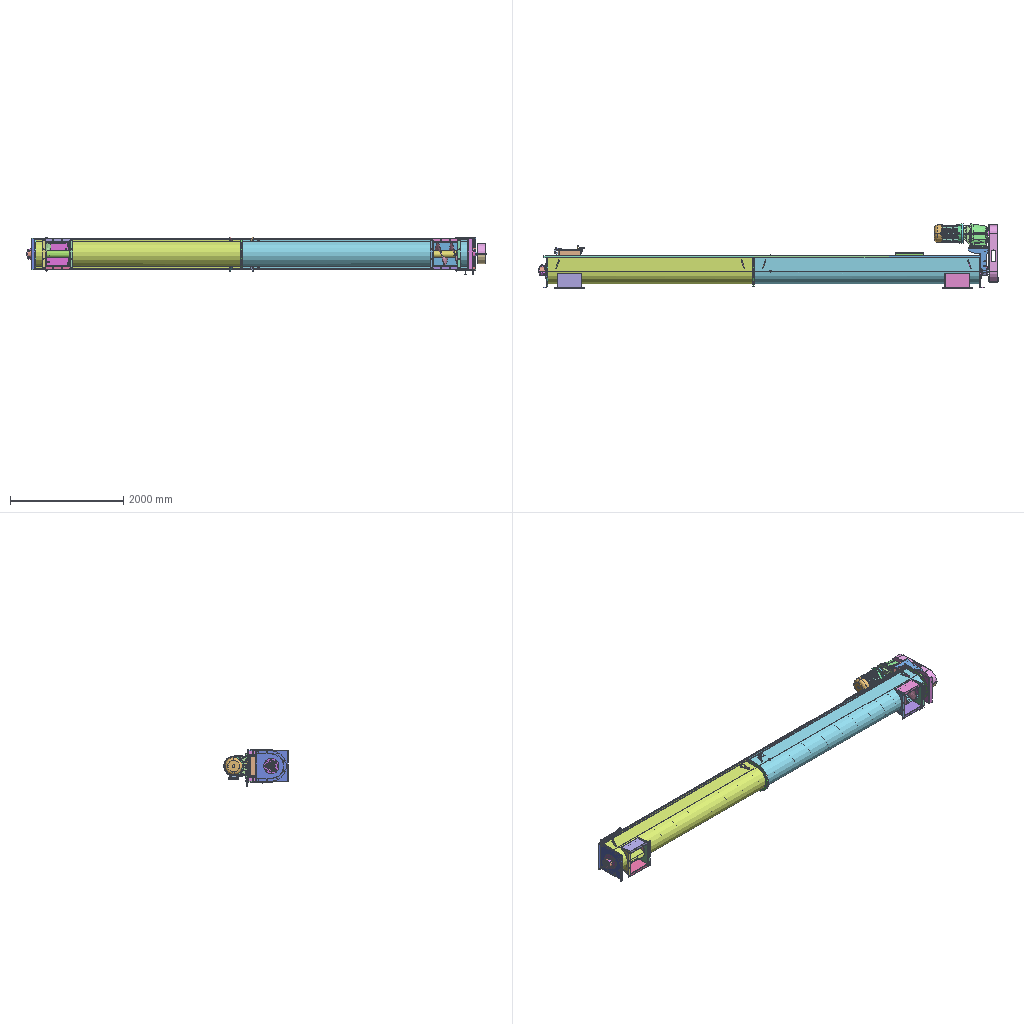Assembly | STEP file | 144 different items | 144 placed | box 8127 x 1140 x 669 mm
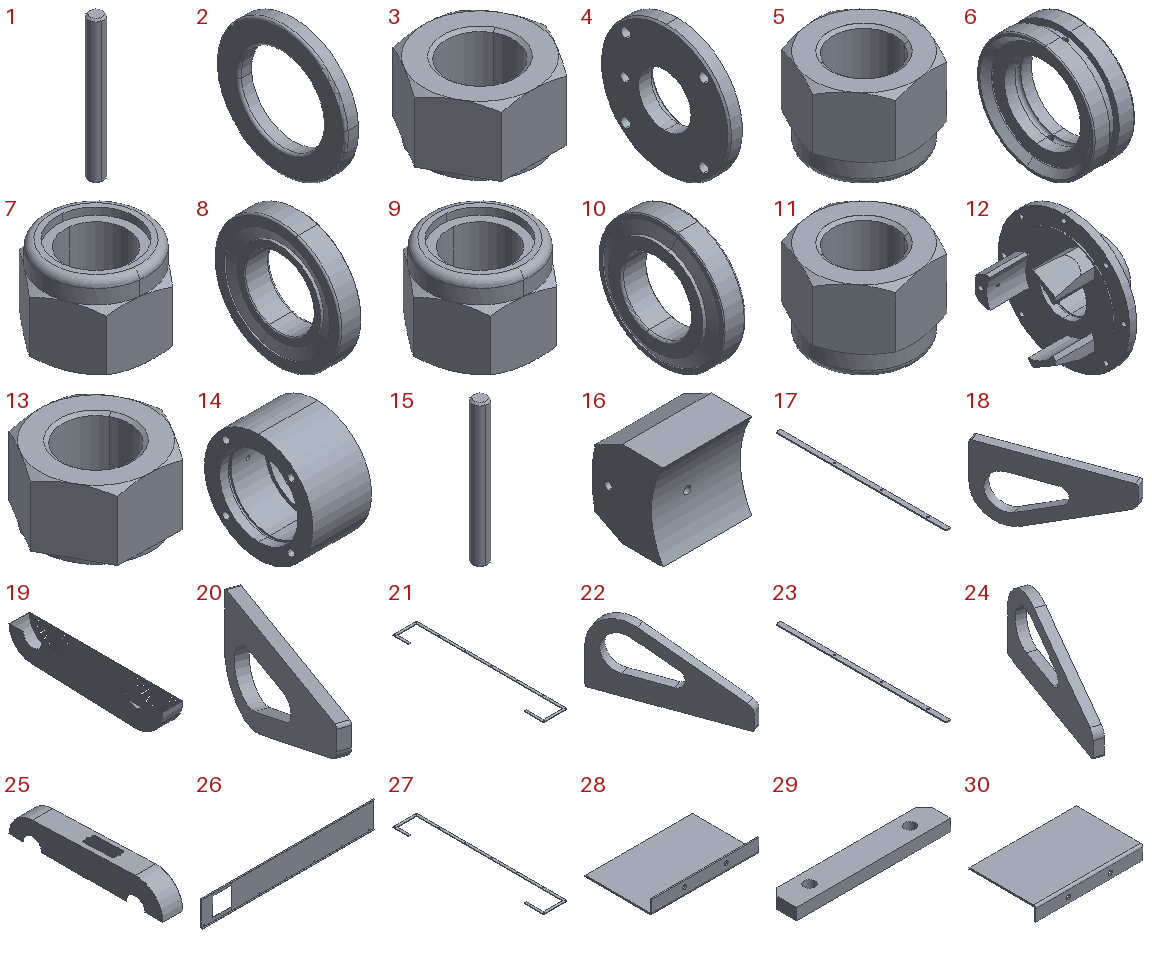Parts list (item | name | quantity | size | volume):
1 | Input 92 | x1 | 16 x 16 x 150 mm | 29975 mm3
2 | Input 21 | x1 | 10 x 100 x 100 mm | 8867 mm3
3 | Input 91 | x1 | 27.707 x 24.281 x 14.8 mm | 4867 mm3
4 | Input 20 | x1 | 25.5 x 153 x 153 mm | 263994 mm3
5 | Input 90 | x1 | 27.478 x 25.596 x 19.1 mm | 5895 mm3
6 | Input 19 | x1 | 35 x 100 x 100 mm | 108578 mm3
7 | Input 89 | x1 | 27.447 x 25.685 x 19.1 mm | 5895 mm3
8 | Input 18 | x1 | 23.75 x 110 x 110 mm | 129421 mm3
9 | Input 88 | x1 | 27.447 x 25.685 x 19.1 mm | 5895 mm3
10 | Input 17 | x1 | 23.75 x 110 x 110 mm | 129421 mm3
11 | Input 87 | x1 | 27.478 x 25.596 x 19.1 mm | 5895 mm3
12 | Input 16 | x1 | 164 x 275 x 275 mm | 1448032 mm3
13 | Input 86 | x1 | 27.707 x 24.281 x 14.8 mm | 4867 mm3
14 | Input 15 | x1 | 82.5 x 153 x 153 mm | 749438 mm3
15 | Input 85 | x1 | 16 x 16 x 150 mm | 29975 mm3
16 | Input 14 | x1 | 62 x 49.538 x 60 mm | 146146 mm3
17 | Input 84 | x1 | 15 x 545 x 3.2 mm | 25854 mm3
18 | Input 13 | x1 | 64.12 x 153.771 x 80 mm | 68539 mm3
19 | Input 83 | x1 | 130 x 990 x 175 mm | 933762 mm3
20 | Input 12 | x1 | 64.12 x 153.771 x 80 mm | 68539 mm3
21 | Input 82 | x1 | 160 x 1020 x 3.2 mm | 71803 mm3
22 | Input 11 | x1 | 64.12 x 153.771 x 80 mm | 68539 mm3
23 | Input 81 | x1 | 15 x 545 x 3.2 mm | 25854 mm3
24 | Input 10 | x1 | 64.12 x 153.771 x 80 mm | 68539 mm3
25 | Input 80 | x1 | 130 x 990 x 175 mm | 933762 mm3
26 | Input 9 | x1 | 3702 x 35 x 559 mm | 9562129 mm3
27 | Input 79 | x1 | 160 x 1020 x 3.2 mm | 71803 mm3
28 | Input 8 | x1 | 425 x 265 x 55 mm | 792268 mm3
29 | Input 78 | x1 | 200 x 35 x 15 mm | 98882 mm3
30 | Input 7 | x1 | 425 x 265 x 55 mm | 792268 mm3
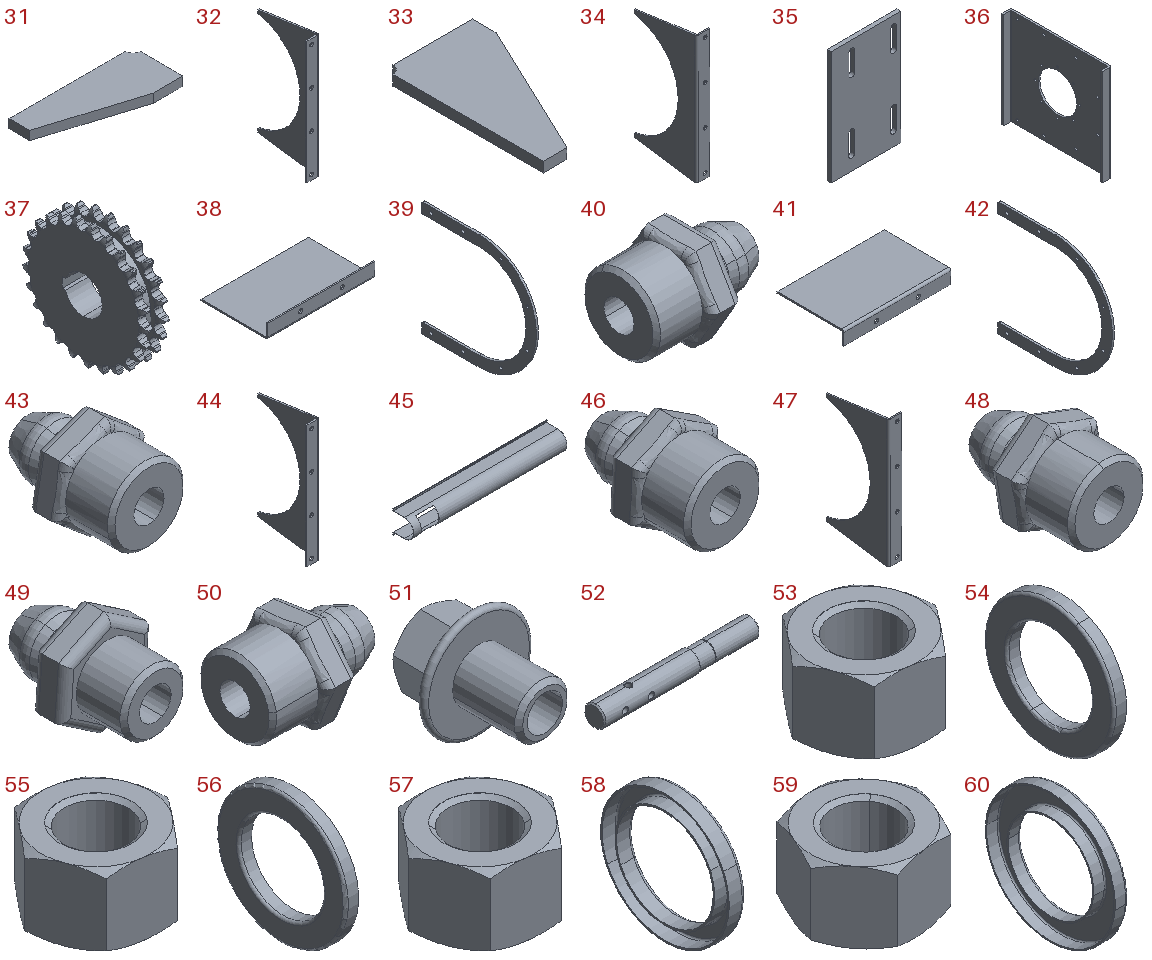31 | Input 77 | x1 | 210 x 85 x 15 mm | 205909 mm3
32 | Input 6 | x1 | 55 x 265 x 540 mm | 579833 mm3
33 | Input 76 | x1 | 130 x 235 x 15 mm | 313909 mm3
34 | Input 5 | x1 | 55 x 265 x 540 mm | 579833 mm3
35 | Input 75 | x1 | 350 x 20 x 570 mm | 3716740 mm3
36 | Input 4 | x1 | 52 x 564 x 540 mm | 3076636 mm3
37 | Input 74 | x1 | 52.8 x 269.775 x 269.908 mm | 2050687 mm3
38 | Input 144 | x1 | 425 x 265 x 55 mm | 792268 mm3
39 | Input 3 | x1 | 10 x 540 x 540 mm | 629249 mm3
40 | Input 73 | x1 | 16 x 12.702 x 11.006 mm | 882.434 mm3
41 | Input 143 | x1 | 425 x 265 x 55 mm | 792268 mm3
42 | Input 2 | x1 | 10 x 540 x 540 mm | 629249 mm3
43 | Input 72 | x1 | 11.955 x 16 x 12.499 mm | 882.434 mm3
44 | Input 142 | x1 | 55 x 265 x 540 mm | 579833 mm3
45 | Input 1 | x1 | 3630 x 490 x 540 mm | 23301858 mm3
46 | Input 71 | x1 | 11.323 x 16 x 12.684 mm | 882.434 mm3
47 | Input 141 | x1 | 55 x 265 x 540 mm | 579833 mm3
48 | Input 70 | x1 | 11.871 x 16 x 12.54 mm | 882.434 mm3
49 | Input 140 | x1 | 11.44 x 16 x 12.667 mm | 712.263 mm3
50 | Input 69 | x1 | 16 x 12.558 x 11.829 mm | 882.434 mm3
51 | Input 139 | x1 | 24.7 x 26.9 x 24.7 mm | 3275 mm3
52 | Input 68 | x1 | 483 x 65 x 65 mm | 1443135 mm3
53 | Input 138 | x1 | 27.415 x 25.769 x 15.9 mm | 5420 mm3
54 | Input 67 | x1 | 10 x 100 x 100 mm | 8867 mm3
55 | Input 137 | x1 | 27.415 x 25.769 x 15.9 mm | 5420 mm3
56 | Input 66 | x1 | 10 x 100 x 100 mm | 8867 mm3
57 | Input 136 | x1 | 27.415 x 25.769 x 15.9 mm | 5420 mm3
58 | Input 65 | x1 | 10 x 80 x 80 mm | 5874 mm3
59 | Input 135 | x1 | 27.465 x 25.634 x 15.9 mm | 5420 mm3
60 | Input 64 | x1 | 10 x 100 x 100 mm | 8867 mm3
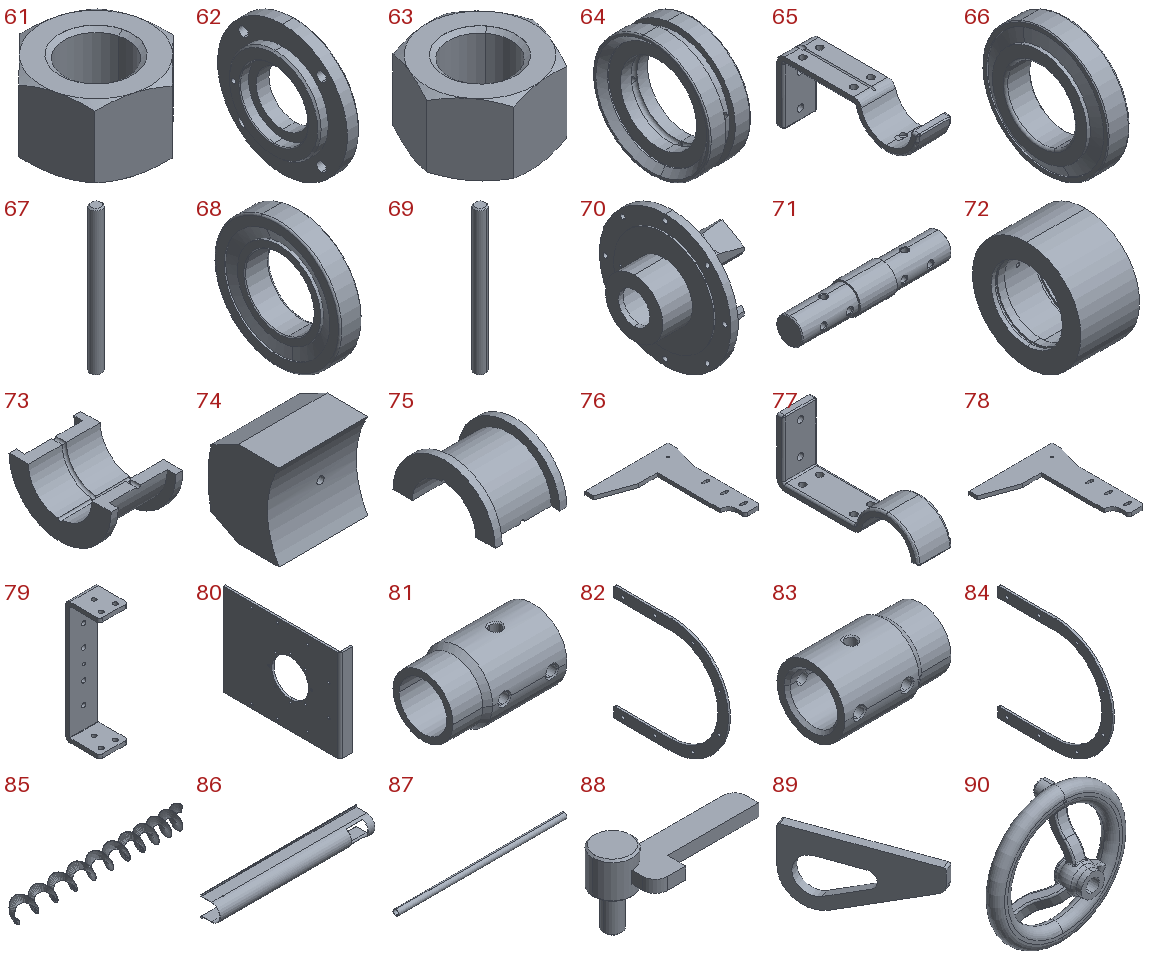61 | Input 134 | x1 | 26.671 x 26.862 x 15.9 mm | 5420 mm3
62 | Input 63 | x1 | 25.5 x 153 x 153 mm | 263994 mm3
63 | Input 133 | x1 | 27.465 x 25.634 x 15.9 mm | 5420 mm3
64 | Input 62 | x1 | 35 x 100 x 100 mm | 108578 mm3
65 | Input 132 | x1 | 80 x 330.779 x 150 mm | 596739 mm3
66 | Input 61 | x1 | 23.75 x 110 x 110 mm | 129421 mm3
67 | Input 131 | x1 | 16 x 16 x 200 mm | 40070 mm3
68 | Input 60 | x1 | 23.75 x 110 x 110 mm | 129421 mm3
69 | Input 130 | x1 | 16 x 16 x 200 mm | 40070 mm3
70 | Input 59 | x1 | 164 x 275 x 275 mm | 1448032 mm3
71 | Input 129 | x1 | 456 x 90 x 90 mm | 2317318 mm3
72 | Input 58 | x1 | 82.5 x 153 x 153 mm | 749438 mm3
73 | Input 128 | x1 | 102 x 145 x 72.5 mm | 300584 mm3
74 | Input 57 | x1 | 62 x 49.538 x 60 mm | 146146 mm3
75 | Input 127 | x1 | 102 x 145 x 72.5 mm | 300584 mm3
76 | Input 56 | x1 | 350 x 420 x 15 mm | 847153 mm3
77 | Input 126 | x1 | 80 x 330.779 x 150 mm | 596739 mm3
78 | Input 55 | x1 | 350 x 420 x 15 mm | 847153 mm3
79 | Input 125 | x1 | 100 x 120 x 430 mm | 862144 mm3
80 | Input 54 | x1 | 75 x 689 x 540 mm | 4383962 mm3
81 | Input 124 | x1 | 185 x 114 x 114 mm | 807255 mm3
82 | Input 53 | x1 | 10 x 540 x 540 mm | 629249 mm3
83 | Input 123 | x1 | 185 x 114 x 114 mm | 807255 mm3
84 | Input 52 | x1 | 10 x 540 x 540 mm | 629249 mm3
85 | Input 122 | x1 | 3576 x 400.387 x 400.36 mm | 9588651 mm3
86 | Input 51 | x1 | 3980 x 490 x 540 mm | 25651911 mm3
87 | Input 121 | x1 | 3309 x 114.3 x 114.3 mm | 6776281 mm3
88 | Input 50 | x1 | 115.97 x 51.074 x 60 mm | 50470 mm3
89 | Input 120 | x1 | 64.12 x 153.771 x 80 mm | 68539 mm3
90 | Input 49 | x1 | 87 x 35.001 x 87 mm | 30093 mm3
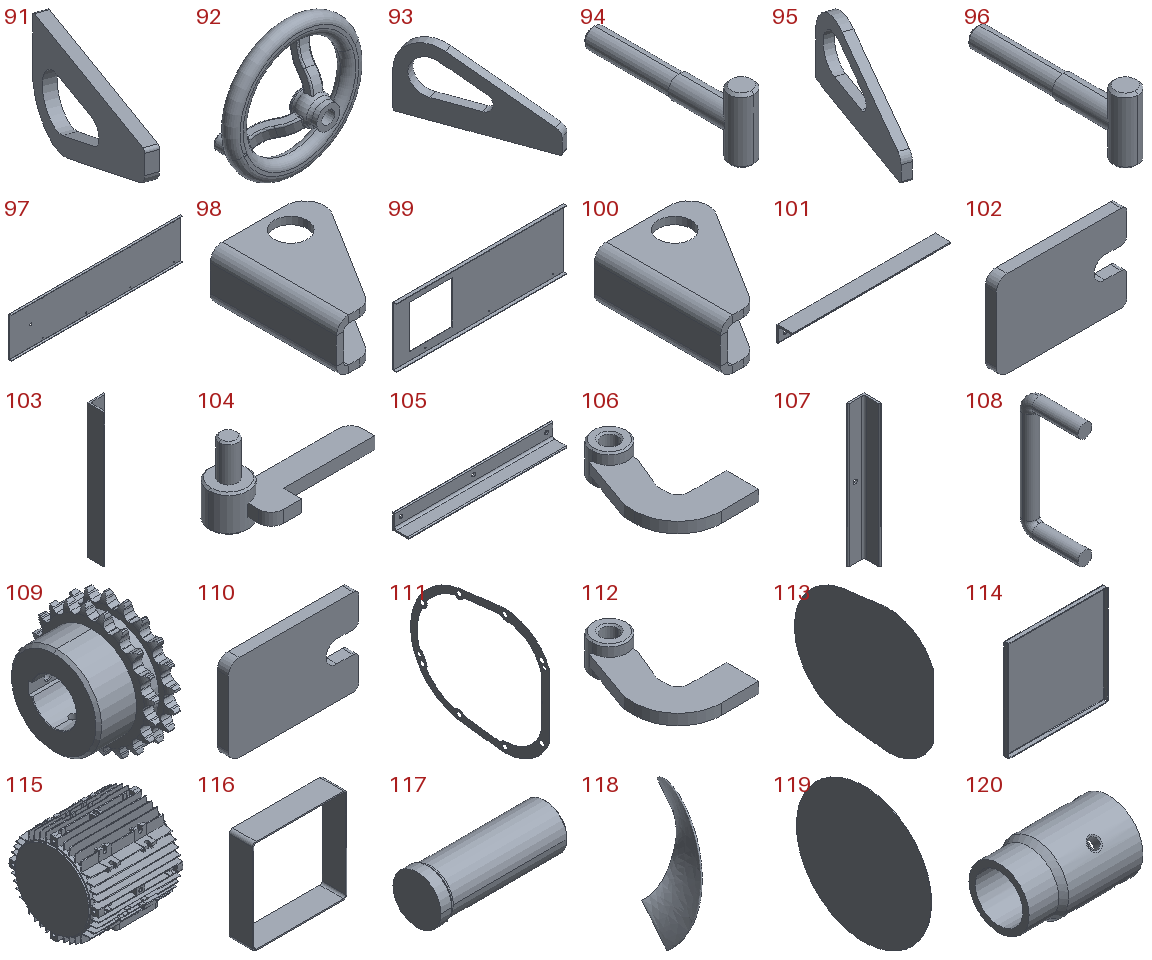91 | Input 119 | x1 | 64.12 x 153.771 x 80 mm | 68539 mm3
92 | Input 48 | x1 | 86.999 x 35.267 x 87 mm | 30093 mm3
93 | Input 118 | x1 | 64.12 x 153.771 x 80 mm | 68539 mm3
94 | Input 47 | x1 | 10 x 65 x 26 mm | 5070 mm3
95 | Input 117 | x1 | 64.12 x 153.771 x 80 mm | 68539 mm3
96 | Input 46 | x1 | 10 x 65.016 x 26 mm | 5070 mm3
97 | Input 116 | x1 | 2395 x 35 x 559 mm | 6649356 mm3
98 | Input 45 | x1 | 30 x 40 x 16 mm | 4444 mm3
99 | Input 115 | x1 | 1600 x 35 x 559 mm | 3723950 mm3
100 | Input 44 | x1 | 30 x 40 x 16 mm | 4444 mm3
101 | Input 114 | x1 | 500 x 50 x 50 mm | 238406 mm3
102 | Input 43 | x1 | 60.015 x 5.178 x 40 mm | 11223 mm3
103 | Input 113 | x1 | 50 x 50 x 400 mm | 191516 mm3
104 | Input 42 | x1 | 115.97 x 51.074 x 60 mm | 50470 mm3
105 | Input 112 | x1 | 500 x 50 x 50 mm | 238406 mm3
106 | Input 41 | x1 | 75.005 x 115.604 x 30 mm | 55549 mm3
107 | Input 111 | x1 | 50 x 50 x 400 mm | 191516 mm3
108 | Input 40 | x1 | 15.178 x 67.522 x 135 mm | 40895 mm3
109 | Input 110 | x1 | 120 x 217.216 x 217.216 mm | 2149688 mm3
110 | Input 39 | x1 | 60.015 x 5.178 x 40 mm | 11223 mm3
111 | Input 109 | x1 | 0.5 x 420 x 377 mm | 13724 mm3
112 | Input 38 | x1 | 75.005 x 115.604 x 30 mm | 55549 mm3
113 | Input 108 | x1 | 0.5 x 420 x 377 mm | 66218 mm3
114 | Input 37 | x1 | 420.785 x 20.607 x 420.745 mm | 642880 mm3
115 | Input 107 | x1 | 300 x 305 x 312.5 mm | 16733446 mm3
116 | Input 36 | x1 | 400 x 100 x 400 mm | 779270 mm3
117 | Input 106 | x1 | 120.5 x 45 x 45 mm | 154941 mm3
118 | Input 35 | x1 | 215.218 x 318.536 x 356.446 mm | 751213 mm3
119 | Input 105 | x1 | 0.5 x 180 x 180 mm | 12723 mm3
120 | Input 34 | x1 | 185 x 114 x 114 mm | 807255 mm3
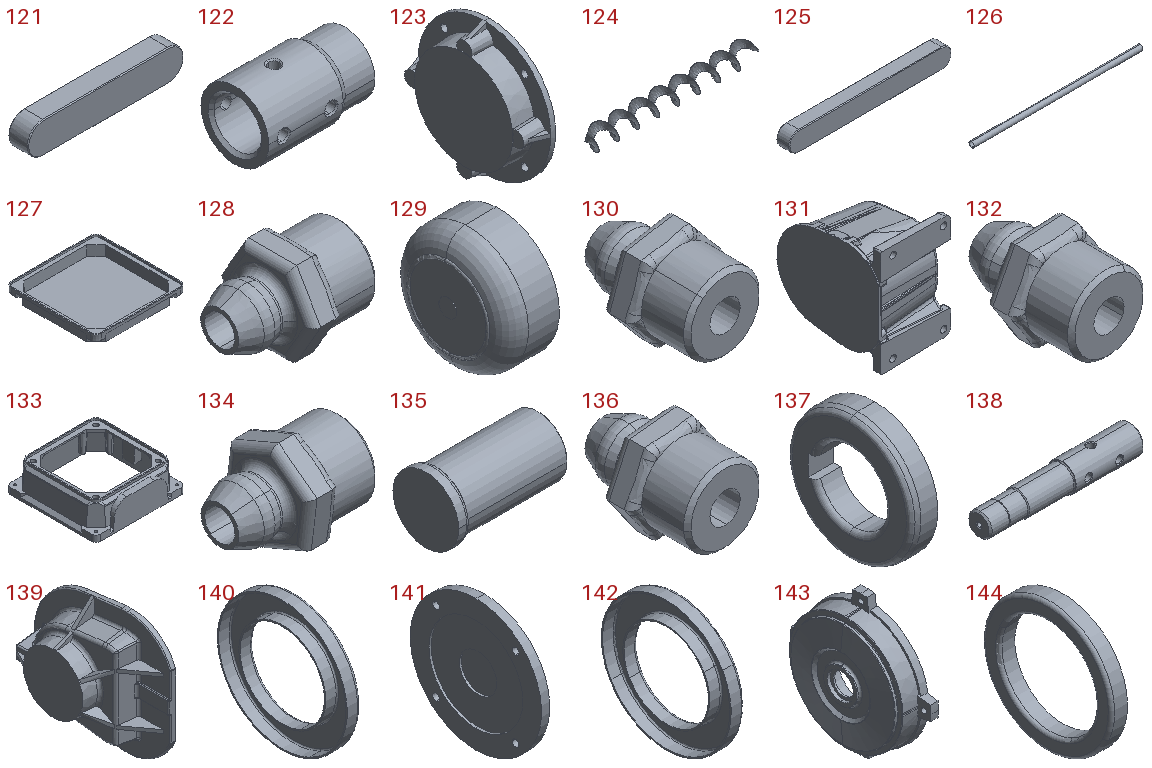121 | Input 104 | x1 | 110 x 14 x 22 mm | 32338 mm3
122 | Input 33 | x1 | 185 x 114 x 114 mm | 807255 mm3
123 | Input 103 | x1 | 73 x 350 x 350 mm | 3966016 mm3
124 | Input 32 | x1 | 3271 x 400.356 x 400.198 mm | 12173770 mm3
125 | Input 102 | x1 | 100 x 8 x 12 mm | 9319 mm3
126 | Input 31 | x1 | 3557 x 114.3 x 114.3 mm | 7284143 mm3
127 | Input 101 | x1 | 186 x 186 x 27 mm | 135182 mm3
128 | Input 30 | x1 | 16 x 12.702 x 11 mm | 882.434 mm3
129 | Input 100 | x1 | 136 x 309 x 309 mm | 181254 mm3
130 | Input 29 | x1 | 12.497 x 16 x 11.958 mm | 882.434 mm3
131 | Input 99 | x1 | 295 x 425 x 439.824 mm | 31332402 mm3
132 | Input 28 | x1 | 12.689 x 16 x 11.273 mm | 882.434 mm3
133 | Input 98 | x1 | 179.5 x 179.5 x 60.5 mm | 241417 mm3
134 | Input 27 | x1 | 16 x 11.686 x 12.609 mm | 882.434 mm3
135 | Input 97 | x1 | 155 x 90 x 90 mm | 763007 mm3
136 | Input 26 | x1 | 12.648 x 16 x 11.535 mm | 882.434 mm3
137 | Input 96 | x1 | 15 x 75 x 75 mm | 43593 mm3
138 | Input 25 | x1 | 393 x 73 x 73 mm | 1345676 mm3
139 | Input 95 | x1 | 130.5 x 420 x 377 mm | 7494076 mm3
140 | Input 24 | x1 | 10 x 100 x 100 mm | 8867 mm3
141 | Input 94 | x1 | 37 x 350 x 350 mm | 2104488 mm3
142 | Input 23 | x1 | 10 x 100 x 100 mm | 8867 mm3
143 | Input 93 | x1 | 63 x 305 x 305 mm | 585521 mm3
144 | Input 22 | x1 | 10 x 80 x 80 mm | 5874 mm3
Placements (level | parent | child | x y z in mm | rotation matrix by rows):
1 | subassembly 2 | Input 92 | -0.0 -0.0 -0.0 | 1 0 0 0 1 0 0 0 1
1 | subassembly 2 | Input 21 | -0.0 -0.0 -0.0 | 1 0 0 0 1 0 0 0 1
1 | subassembly 2 | Input 91 | -0.0 -0.0 -0.0 | 1 0 0 0 1 0 0 0 1
1 | subassembly 2 | Input 20 | -0.0 -0.0 -0.0 | 1 0 0 0 1 0 0 0 1
1 | subassembly 2 | Input 90 | -0.0 -0.0 -0.0 | 1 0 0 0 1 0 0 0 1
1 | subassembly 2 | Input 19 | -0.0 -0.0 -0.0 | 1 0 0 0 1 0 0 0 1
1 | subassembly 2 | Input 89 | -0.0 -0.0 -0.0 | 1 0 0 0 1 0 0 0 1
1 | subassembly 2 | Input 18 | -0.0 -0.0 -0.0 | 1 0 0 0 1 0 0 0 1
1 | subassembly 2 | Input 88 | -0.0 -0.0 -0.0 | 1 0 0 0 1 0 0 0 1
1 | subassembly 2 | Input 17 | -0.0 -0.0 -0.0 | 1 0 0 0 1 0 0 0 1
1 | subassembly 2 | Input 87 | -0.0 -0.0 -0.0 | 1 0 0 0 1 0 0 0 1
1 | subassembly 2 | Input 16 | -0.0 -0.0 -0.0 | 1 0 0 0 1 0 0 0 1
1 | subassembly 2 | Input 86 | -0.0 -0.0 -0.0 | 1 0 0 0 1 0 0 0 1
1 | subassembly 2 | Input 15 | -0.0 -0.0 -0.0 | 1 0 0 0 1 0 0 0 1
1 | subassembly 2 | Input 85 | -0.0 -0.0 -0.0 | 1 0 0 0 1 0 0 0 1
1 | subassembly 2 | Input 14 | -0.0 -0.0 -0.0 | 1 0 0 0 1 0 0 0 1
1 | subassembly 2 | Input 84 | -0.0 -0.0 -0.0 | 1 0 0 0 1 0 0 0 1
1 | subassembly 2 | Input 13 | -0.0 -0.0 -0.0 | 1 0 0 0 1 0 0 0 1
1 | subassembly 2 | Input 83 | -0.0 -0.0 -0.0 | 1 0 0 0 1 0 0 0 1
1 | subassembly 2 | Input 12 | -0.0 -0.0 -0.0 | 1 0 0 0 1 0 0 0 1
1 | subassembly 2 | Input 82 | -0.0 -0.0 -0.0 | 1 0 0 0 1 0 0 0 1
1 | subassembly 2 | Input 11 | -0.0 -0.0 -0.0 | 1 0 0 0 1 0 0 0 1
1 | subassembly 2 | Input 81 | -0.0 -0.0 -0.0 | 1 0 0 0 1 0 0 0 1
1 | subassembly 2 | Input 10 | -0.0 -0.0 -0.0 | 1 0 0 0 1 0 0 0 1
1 | subassembly 2 | Input 80 | -0.0 -0.0 -0.0 | 1 0 0 0 1 0 0 0 1
1 | subassembly 2 | Input 9 | -0.0 -0.0 -0.0 | 1 0 0 0 1 0 0 0 1
1 | subassembly 2 | Input 79 | -0.0 -0.0 -0.0 | 1 0 0 0 1 0 0 0 1
1 | subassembly 2 | Input 8 | -0.0 -0.0 -0.0 | 1 0 0 0 1 0 0 0 1
1 | subassembly 2 | Input 78 | -0.0 -0.0 -0.0 | 1 0 0 0 1 0 0 0 1
1 | subassembly 2 | Input 7 | -0.0 -0.0 -0.0 | 1 0 0 0 1 0 0 0 1
1 | subassembly 2 | Input 77 | -0.0 -0.0 -0.0 | 1 0 0 0 1 0 0 0 1
1 | subassembly 2 | Input 6 | -0.0 -0.0 -0.0 | 1 0 0 0 1 0 0 0 1
1 | subassembly 2 | Input 76 | -0.0 -0.0 -0.0 | 1 0 0 0 1 0 0 0 1
1 | subassembly 2 | Input 5 | -0.0 -0.0 -0.0 | 1 0 0 0 1 0 0 0 1
1 | subassembly 2 | Input 75 | -0.0 -0.0 -0.0 | 1 0 0 0 1 0 0 0 1
1 | subassembly 2 | Input 4 | -0.0 -0.0 -0.0 | 1 0 0 0 1 0 0 0 1
1 | subassembly 2 | Input 74 | -0.0 -0.0 -0.0 | 1 0 0 0 1 0 0 0 1
1 | subassembly 2 | Input 144 | -0.0 -0.0 -0.0 | 1 0 0 0 1 0 0 0 1
1 | subassembly 2 | Input 3 | -0.0 -0.0 -0.0 | 1 0 0 0 1 0 0 0 1
1 | subassembly 2 | Input 73 | -0.0 -0.0 -0.0 | 1 0 0 0 1 0 0 0 1
1 | subassembly 2 | Input 143 | -0.0 -0.0 -0.0 | 1 0 0 0 1 0 0 0 1
1 | subassembly 2 | Input 2 | -0.0 -0.0 -0.0 | 1 0 0 0 1 0 0 0 1
1 | subassembly 2 | Input 72 | -0.0 -0.0 -0.0 | 1 0 0 0 1 0 0 0 1
1 | subassembly 2 | Input 142 | -0.0 -0.0 -0.0 | 1 0 0 0 1 0 0 0 1
1 | subassembly 2 | Input 1 | -0.0 -0.0 -0.0 | 1 0 0 0 1 0 0 0 1
1 | subassembly 2 | Input 71 | -0.0 -0.0 -0.0 | 1 0 0 0 1 0 0 0 1
1 | subassembly 2 | Input 141 | -0.0 -0.0 -0.0 | 1 0 0 0 1 0 0 0 1
1 | subassembly 2 | Input 70 | -0.0 -0.0 -0.0 | 1 0 0 0 1 0 0 0 1
1 | subassembly 2 | Input 140 | -0.0 -0.0 -0.0 | 1 0 0 0 1 0 0 0 1
1 | subassembly 2 | Input 69 | -0.0 -0.0 -0.0 | 1 0 0 0 1 0 0 0 1
1 | subassembly 2 | Input 139 | -0.0 -0.0 -0.0 | 1 0 0 0 1 0 0 0 1
1 | subassembly 2 | Input 68 | -0.0 -0.0 -0.0 | 1 0 0 0 1 0 0 0 1
1 | subassembly 2 | Input 138 | -0.0 -0.0 -0.0 | 1 0 0 0 1 0 0 0 1
1 | subassembly 2 | Input 67 | -0.0 -0.0 -0.0 | 1 0 0 0 1 0 0 0 1
1 | subassembly 2 | Input 137 | -0.0 -0.0 -0.0 | 1 0 0 0 1 0 0 0 1
1 | subassembly 2 | Input 66 | -0.0 -0.0 -0.0 | 1 0 0 0 1 0 0 0 1
1 | subassembly 2 | Input 136 | -0.0 -0.0 -0.0 | 1 0 0 0 1 0 0 0 1
1 | subassembly 2 | Input 65 | -0.0 -0.0 -0.0 | 1 0 0 0 1 0 0 0 1
1 | subassembly 2 | Input 135 | -0.0 -0.0 -0.0 | 1 0 0 0 1 0 0 0 1
1 | subassembly 2 | Input 64 | -0.0 -0.0 -0.0 | 1 0 0 0 1 0 0 0 1
1 | subassembly 2 | Input 134 | -0.0 -0.0 -0.0 | 1 0 0 0 1 0 0 0 1
1 | subassembly 2 | Input 63 | -0.0 -0.0 -0.0 | 1 0 0 0 1 0 0 0 1
1 | subassembly 2 | Input 133 | -0.0 -0.0 -0.0 | 1 0 0 0 1 0 0 0 1
1 | subassembly 2 | Input 62 | -0.0 -0.0 -0.0 | 1 0 0 0 1 0 0 0 1
1 | subassembly 2 | Input 132 | -0.0 -0.0 -0.0 | 1 0 0 0 1 0 0 0 1
1 | subassembly 2 | Input 61 | -0.0 -0.0 -0.0 | 1 0 0 0 1 0 0 0 1
1 | subassembly 2 | Input 131 | -0.0 -0.0 -0.0 | 1 0 0 0 1 0 0 0 1
1 | subassembly 2 | Input 60 | -0.0 -0.0 -0.0 | 1 0 0 0 1 0 0 0 1
1 | subassembly 2 | Input 130 | -0.0 -0.0 -0.0 | 1 0 0 0 1 0 0 0 1
1 | subassembly 2 | Input 59 | -0.0 -0.0 -0.0 | 1 0 0 0 1 0 0 0 1
1 | subassembly 2 | Input 129 | -0.0 -0.0 -0.0 | 1 0 0 0 1 0 0 0 1
1 | subassembly 2 | Input 58 | -0.0 -0.0 -0.0 | 1 0 0 0 1 0 0 0 1
1 | subassembly 2 | Input 128 | -0.0 -0.0 -0.0 | 1 0 0 0 1 0 0 0 1
1 | subassembly 2 | Input 57 | -0.0 -0.0 -0.0 | 1 0 0 0 1 0 0 0 1
1 | subassembly 2 | Input 127 | -0.0 -0.0 -0.0 | 1 0 0 0 1 0 0 0 1
1 | subassembly 2 | Input 56 | -0.0 -0.0 -0.0 | 1 0 0 0 1 0 0 0 1
1 | subassembly 2 | Input 126 | -0.0 -0.0 -0.0 | 1 0 0 0 1 0 0 0 1
1 | subassembly 2 | Input 55 | -0.0 -0.0 -0.0 | 1 0 0 0 1 0 0 0 1
1 | subassembly 2 | Input 125 | -0.0 -0.0 -0.0 | 1 0 0 0 1 0 0 0 1
1 | subassembly 2 | Input 54 | -0.0 -0.0 -0.0 | 1 0 0 0 1 0 0 0 1
1 | subassembly 2 | Input 124 | -0.0 -0.0 -0.0 | 1 0 0 0 1 0 0 0 1
1 | subassembly 2 | Input 53 | -0.0 -0.0 -0.0 | 1 0 0 0 1 0 0 0 1
1 | subassembly 2 | Input 123 | -0.0 -0.0 -0.0 | 1 0 0 0 1 0 0 0 1
1 | subassembly 2 | Input 52 | -0.0 -0.0 -0.0 | 1 0 0 0 1 0 0 0 1
1 | subassembly 2 | Input 122 | -0.0 -0.0 -0.0 | 1 0 0 0 1 0 0 0 1
1 | subassembly 2 | Input 51 | -0.0 -0.0 -0.0 | 1 0 0 0 1 0 0 0 1
1 | subassembly 2 | Input 121 | -0.0 -0.0 -0.0 | 1 0 0 0 1 0 0 0 1
1 | subassembly 2 | Input 50 | -0.0 -0.0 -0.0 | 1 0 0 0 1 0 0 0 1
1 | subassembly 2 | Input 120 | -0.0 -0.0 -0.0 | 1 0 0 0 1 0 0 0 1
1 | subassembly 2 | Input 49 | -0.0 -0.0 -0.0 | 1 0 0 0 1 0 0 0 1
1 | subassembly 2 | Input 119 | -0.0 -0.0 -0.0 | 1 0 0 0 1 0 0 0 1
1 | subassembly 2 | Input 48 | -0.0 -0.0 -0.0 | 1 0 0 0 1 0 0 0 1
1 | subassembly 2 | Input 118 | -0.0 -0.0 -0.0 | 1 0 0 0 1 0 0 0 1
1 | subassembly 2 | Input 47 | -0.0 -0.0 -0.0 | 1 0 0 0 1 0 0 0 1
1 | subassembly 2 | Input 117 | -0.0 -0.0 -0.0 | 1 0 0 0 1 0 0 0 1
1 | subassembly 2 | Input 46 | -0.0 -0.0 -0.0 | 1 0 0 0 1 0 0 0 1
1 | subassembly 2 | Input 116 | -0.0 -0.0 -0.0 | 1 0 0 0 1 0 0 0 1
1 | subassembly 2 | Input 45 | -0.0 -0.0 -0.0 | 1 0 0 0 1 0 0 0 1
1 | subassembly 2 | Input 115 | -0.0 -0.0 -0.0 | 1 0 0 0 1 0 0 0 1
1 | subassembly 2 | Input 44 | -0.0 -0.0 -0.0 | 1 0 0 0 1 0 0 0 1
1 | subassembly 2 | Input 114 | -0.0 -0.0 -0.0 | 1 0 0 0 1 0 0 0 1
1 | subassembly 2 | Input 43 | -0.0 -0.0 -0.0 | 1 0 0 0 1 0 0 0 1
1 | subassembly 2 | Input 113 | -0.0 -0.0 -0.0 | 1 0 0 0 1 0 0 0 1
1 | subassembly 2 | Input 42 | -0.0 -0.0 -0.0 | 1 0 0 0 1 0 0 0 1
1 | subassembly 2 | Input 112 | -0.0 -0.0 -0.0 | 1 0 0 0 1 0 0 0 1
1 | subassembly 2 | Input 41 | -0.0 -0.0 -0.0 | 1 0 0 0 1 0 0 0 1
1 | subassembly 2 | Input 111 | -0.0 -0.0 -0.0 | 1 0 0 0 1 0 0 0 1
1 | subassembly 2 | Input 40 | -0.0 -0.0 -0.0 | 1 0 0 0 1 0 0 0 1
1 | subassembly 2 | Input 110 | -0.0 -0.0 -0.0 | 1 0 0 0 1 0 0 0 1
1 | subassembly 2 | Input 39 | -0.0 -0.0 -0.0 | 1 0 0 0 1 0 0 0 1
1 | subassembly 2 | Input 109 | -0.0 -0.0 -0.0 | 1 0 0 0 1 0 0 0 1
1 | subassembly 2 | Input 38 | -0.0 -0.0 -0.0 | 1 0 0 0 1 0 0 0 1
1 | subassembly 2 | Input 108 | -0.0 -0.0 -0.0 | 1 0 0 0 1 0 0 0 1
1 | subassembly 2 | Input 37 | -0.0 -0.0 -0.0 | 1 0 0 0 1 0 0 0 1
1 | subassembly 2 | Input 107 | -0.0 -0.0 -0.0 | 1 0 0 0 1 0 0 0 1
1 | subassembly 2 | Input 36 | -0.0 -0.0 -0.0 | 1 0 0 0 1 0 0 0 1
1 | subassembly 2 | Input 106 | -0.0 -0.0 -0.0 | 1 0 0 0 1 0 0 0 1
1 | subassembly 2 | Input 35 | -0.0 -0.0 -0.0 | 1 0 0 0 1 0 0 0 1
1 | subassembly 2 | Input 105 | -0.0 -0.0 -0.0 | 1 0 0 0 1 0 0 0 1
1 | subassembly 2 | Input 34 | -0.0 -0.0 -0.0 | 1 0 0 0 1 0 0 0 1
1 | subassembly 2 | Input 104 | -0.0 -0.0 -0.0 | 1 0 0 0 1 0 0 0 1
1 | subassembly 2 | Input 33 | -0.0 -0.0 -0.0 | 1 0 0 0 1 0 0 0 1
1 | subassembly 2 | Input 103 | -0.0 -0.0 -0.0 | 1 0 0 0 1 0 0 0 1
1 | subassembly 2 | Input 32 | -0.0 -0.0 -0.0 | 1 0 0 0 1 0 0 0 1
1 | subassembly 2 | Input 102 | -0.0 -0.0 -0.0 | 1 0 0 0 1 0 0 0 1
1 | subassembly 2 | Input 31 | -0.0 -0.0 -0.0 | 1 0 0 0 1 0 0 0 1
1 | subassembly 2 | Input 101 | -0.0 -0.0 -0.0 | 1 0 0 0 1 0 0 0 1
1 | subassembly 2 | Input 30 | -0.0 -0.0 -0.0 | 1 0 0 0 1 0 0 0 1
1 | subassembly 2 | Input 100 | -0.0 -0.0 -0.0 | 1 0 0 0 1 0 0 0 1
1 | subassembly 2 | Input 29 | -0.0 -0.0 -0.0 | 1 0 0 0 1 0 0 0 1
1 | subassembly 2 | Input 99 | -0.0 -0.0 -0.0 | 1 0 0 0 1 0 0 0 1
1 | subassembly 2 | Input 28 | -0.0 -0.0 -0.0 | 1 0 0 0 1 0 0 0 1
1 | subassembly 2 | Input 98 | -0.0 -0.0 -0.0 | 1 0 0 0 1 0 0 0 1
1 | subassembly 2 | Input 27 | -0.0 -0.0 -0.0 | 1 0 0 0 1 0 0 0 1
1 | subassembly 2 | Input 97 | -0.0 -0.0 -0.0 | 1 0 0 0 1 0 0 0 1
1 | subassembly 2 | Input 26 | -0.0 -0.0 -0.0 | 1 0 0 0 1 0 0 0 1
1 | subassembly 2 | Input 96 | -0.0 -0.0 -0.0 | 1 0 0 0 1 0 0 0 1
1 | subassembly 2 | Input 25 | -0.0 -0.0 -0.0 | 1 0 0 0 1 0 0 0 1
1 | subassembly 2 | Input 95 | -0.0 -0.0 -0.0 | 1 0 0 0 1 0 0 0 1
1 | subassembly 2 | Input 24 | -0.0 -0.0 -0.0 | 1 0 0 0 1 0 0 0 1
1 | subassembly 2 | Input 94 | -0.0 -0.0 -0.0 | 1 0 0 0 1 0 0 0 1
1 | subassembly 2 | Input 23 | -0.0 -0.0 -0.0 | 1 0 0 0 1 0 0 0 1
1 | subassembly 2 | Input 93 | -0.0 -0.0 -0.0 | 1 0 0 0 1 0 0 0 1
1 | subassembly 2 | Input 22 | -0.0 -0.0 -0.0 | 1 0 0 0 1 0 0 0 1